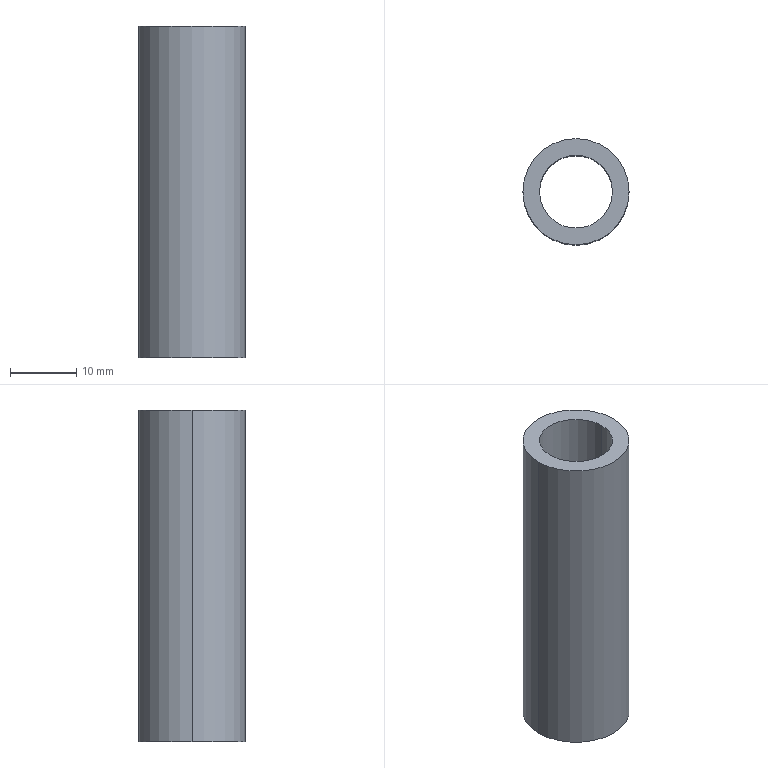Part | SolidWorks | features BaseBody 1 | 1 solid | 6 faces | box 16 x 16 x 50 mm | volume 5301 mm3 | cylinder 4 | plane 2 | commonest cylinder face diameters 11 x2 16 x2
STEP:
#1=CARTESIAN_POINT('',(-5.5,0.,-50.));
#2=VERTEX_POINT('',#1);
#3=CARTESIAN_POINT('',(-5.5,0.,0.));
#4=VERTEX_POINT('',#3);
#5=CARTESIAN_POINT('',(-5.5,0.,-50.));
#6=DIRECTION('',(0.,0.,1.));
#7=VECTOR('',#6,1000.);
#8=LINE('',#5,#7);
#9=EDGE_CURVE('',#2,#4,#8,.T.);
#10=ORIENTED_EDGE('',*,*,#9,.F.);
#11=CARTESIAN_POINT('',(5.5,0.,-50.));
#12=VERTEX_POINT('',#11);
#13=CARTESIAN_POINT('',(0.,0.,-50.));
#14=DIRECTION('',(0.,0.,1.));
#15=DIRECTION('',(1.,0.,0.));
#16=AXIS2_PLACEMENT_3D('',#13,#14,#15);
#17=CIRCLE('',#16,5.5);
#18=EDGE_CURVE('',#12,#2,#17,.T.);
#19=ORIENTED_EDGE('',*,*,#18,.F.);
#20=CARTESIAN_POINT('',(5.5,0.,0.));
#21=VERTEX_POINT('',#20);
#22=CARTESIAN_POINT('',(5.5,0.,-50.));
#23=DIRECTION('',(0.,0.,1.));
#24=VECTOR('',#23,1000.);
#25=LINE('',#22,#24);
#26=EDGE_CURVE('',#12,#21,#25,.T.);
#27=ORIENTED_EDGE('',*,*,#26,.T.);
#28=CARTESIAN_POINT('',(0.,0.,0.));
#29=DIRECTION('',(0.,0.,1.));
#30=DIRECTION('',(1.,0.,0.));
#31=AXIS2_PLACEMENT_3D('',#28,#29,#30);
#32=CIRCLE('',#31,5.5);
#33=EDGE_CURVE('',#21,#4,#32,.T.);
#34=ORIENTED_EDGE('',*,*,#33,.T.);
#35=EDGE_LOOP('',(#10,#19,#27,#34));
#36=FACE_OUTER_BOUND('',#35,.T.);
#37=CARTESIAN_POINT('',(0.,0.,-50.));
#38=DIRECTION('',(0.,0.,1.));
#39=DIRECTION('',(1.,0.,0.));
#40=AXIS2_PLACEMENT_3D('',#37,#38,#39);
#41=CYLINDRICAL_SURFACE('',#40,5.5);
#42=ADVANCED_FACE('',(#36),#41,.F.);
#43=ORIENTED_EDGE('',*,*,#33,.F.);
#44=CARTESIAN_POINT('',(0.,0.,0.));
#45=DIRECTION('',(0.,0.,1.));
#46=DIRECTION('',(1.,0.,0.));
#47=AXIS2_PLACEMENT_3D('',#44,#45,#46);
#48=CIRCLE('',#47,5.5);
#49=EDGE_CURVE('',#4,#21,#48,.T.);
#50=ORIENTED_EDGE('',*,*,#49,.F.);
#51=EDGE_LOOP('',(#43,#50));
#52=FACE_BOUND('',#51,.T.);
#53=CARTESIAN_POINT('',(8.,0.,0.));
#54=VERTEX_POINT('',#53);
#55=CARTESIAN_POINT('',(-8.,0.,0.));
#56=VERTEX_POINT('',#55);
#57=CARTESIAN_POINT('',(0.,0.,0.));
#58=DIRECTION('',(0.,0.,1.));
#59=DIRECTION('',(1.,0.,0.));
#60=AXIS2_PLACEMENT_3D('',#57,#58,#59);
#61=CIRCLE('',#60,8.);
#62=EDGE_CURVE('',#54,#56,#61,.T.);
#63=ORIENTED_EDGE('',*,*,#62,.T.);
#64=CARTESIAN_POINT('',(0.,0.,0.));
#65=DIRECTION('',(0.,0.,1.));
#66=DIRECTION('',(1.,0.,0.));
#67=AXIS2_PLACEMENT_3D('',#64,#65,#66);
#68=CIRCLE('',#67,8.);
#69=EDGE_CURVE('',#56,#54,#68,.T.);
#70=ORIENTED_EDGE('',*,*,#69,.T.);
#71=EDGE_LOOP('',(#63,#70));
#72=FACE_OUTER_BOUND('',#71,.T.);
#73=CARTESIAN_POINT('',(0.,0.,0.));
#74=DIRECTION('',(0.,0.,1.));
#75=DIRECTION('',(1.,0.,0.));
#76=AXIS2_PLACEMENT_3D('',#73,#74,#75);
#77=PLANE('',#76);
#78=ADVANCED_FACE('',(#52,#72),#77,.T.);
#79=ORIENTED_EDGE('',*,*,#18,.T.);
#80=CARTESIAN_POINT('',(0.,0.,-50.));
#81=DIRECTION('',(0.,0.,1.));
#82=DIRECTION('',(1.,0.,0.));
#83=AXIS2_PLACEMENT_3D('',#80,#81,#82);
#84=CIRCLE('',#83,5.5);
#85=EDGE_CURVE('',#2,#12,#84,.T.);
#86=ORIENTED_EDGE('',*,*,#85,.T.);
#87=EDGE_LOOP('',(#79,#86));
#88=FACE_BOUND('',#87,.T.);
#89=CARTESIAN_POINT('',(8.,0.,-50.));
#90=VERTEX_POINT('',#89);
#91=CARTESIAN_POINT('',(-8.,0.,-50.));
#92=VERTEX_POINT('',#91);
#93=CARTESIAN_POINT('',(0.,0.,-50.));
#94=DIRECTION('',(0.,0.,1.));
#95=DIRECTION('',(1.,0.,0.));
#96=AXIS2_PLACEMENT_3D('',#93,#94,#95);
#97=CIRCLE('',#96,8.);
#98=EDGE_CURVE('',#90,#92,#97,.T.);
#99=ORIENTED_EDGE('',*,*,#98,.F.);
#100=CARTESIAN_POINT('',(0.,0.,-50.));
#101=DIRECTION('',(0.,0.,1.));
#102=DIRECTION('',(1.,0.,0.));
#103=AXIS2_PLACEMENT_3D('',#100,#101,#102);
#104=CIRCLE('',#103,8.);
#105=EDGE_CURVE('',#92,#90,#104,.T.);
#106=ORIENTED_EDGE('',*,*,#105,.F.);
#107=EDGE_LOOP('',(#99,#106));
#108=FACE_OUTER_BOUND('',#107,.T.);
#109=CARTESIAN_POINT('',(0.,0.,-50.));
#110=DIRECTION('',(0.,0.,1.));
#111=DIRECTION('',(1.,0.,0.));
#112=AXIS2_PLACEMENT_3D('',#109,#110,#111);
#113=PLANE('',#112);
#114=ADVANCED_FACE('',(#88,#108),#113,.F.);
#115=CARTESIAN_POINT('',(-8.,0.,-50.));
#116=DIRECTION('',(0.,0.,1.));
#117=VECTOR('',#116,1000.);
#118=LINE('',#115,#117);
#119=EDGE_CURVE('',#92,#56,#118,.T.);
#120=ORIENTED_EDGE('',*,*,#119,.F.);
#121=ORIENTED_EDGE('',*,*,#105,.T.);
#122=CARTESIAN_POINT('',(8.,0.,-50.));
#123=DIRECTION('',(0.,0.,1.));
#124=VECTOR('',#123,1000.);
#125=LINE('',#122,#124);
#126=EDGE_CURVE('',#90,#54,#125,.T.);
#127=ORIENTED_EDGE('',*,*,#126,.T.);
#128=ORIENTED_EDGE('',*,*,#69,.F.);
#129=EDGE_LOOP('',(#120,#121,#127,#128));
#130=FACE_OUTER_BOUND('',#129,.T.);
#131=CARTESIAN_POINT('',(0.,0.,-50.));
#132=DIRECTION('',(0.,0.,1.));
#133=DIRECTION('',(1.,0.,0.));
#134=AXIS2_PLACEMENT_3D('',#131,#132,#133);
#135=CYLINDRICAL_SURFACE('',#134,8.);
#136=ADVANCED_FACE('',(#130),#135,.T.);
#137=ORIENTED_EDGE('',*,*,#98,.T.);
#138=ORIENTED_EDGE('',*,*,#119,.T.);
#139=ORIENTED_EDGE('',*,*,#62,.F.);
#140=ORIENTED_EDGE('',*,*,#126,.F.);
#141=EDGE_LOOP('',(#137,#138,#139,#140));
#142=FACE_OUTER_BOUND('',#141,.T.);
#143=CARTESIAN_POINT('',(0.,0.,-50.));
#144=DIRECTION('',(0.,0.,1.));
#145=DIRECTION('',(1.,0.,0.));
#146=AXIS2_PLACEMENT_3D('',#143,#144,#145);
#147=CYLINDRICAL_SURFACE('',#146,8.);
#148=ADVANCED_FACE('',(#142),#147,.T.);
#149=ORIENTED_EDGE('',*,*,#85,.F.);
#150=ORIENTED_EDGE('',*,*,#9,.T.);
#151=ORIENTED_EDGE('',*,*,#49,.T.);
#152=ORIENTED_EDGE('',*,*,#26,.F.);
#153=EDGE_LOOP('',(#149,#150,#151,#152));
#154=FACE_OUTER_BOUND('',#153,.T.);
#155=CARTESIAN_POINT('',(0.,0.,-50.));
#156=DIRECTION('',(0.,0.,1.));
#157=DIRECTION('',(1.,0.,0.));
#158=AXIS2_PLACEMENT_3D('',#155,#156,#157);
#159=CYLINDRICAL_SURFACE('',#158,5.5);
#160=ADVANCED_FACE('',(#154),#159,.F.);
#161=CLOSED_SHELL('',(#42,#78,#114,#136,#148,#160));
#162=MANIFOLD_SOLID_BREP('',#161);
#163=CARTESIAN_POINT('',(0.,0.,0.));
#164=DIRECTION('',(0.,0.,1.));
#165=DIRECTION('',(1.,0.,0.));
#166=AXIS2_PLACEMENT_3D('',#163,#164,#165);
#167=(LENGTH_UNIT()NAMED_UNIT(*)SI_UNIT(.MILLI.,.METRE.));
#168=UNCERTAINTY_MEASURE_WITH_UNIT(LENGTH_MEASURE(0.00001),#167,'','');
#169=(NAMED_UNIT(*)PLANE_ANGLE_UNIT()SI_UNIT($,.RADIAN.));
#170=(NAMED_UNIT(*)SI_UNIT($,.STERADIAN.)SOLID_ANGLE_UNIT());
#171=(GEOMETRIC_REPRESENTATION_CONTEXT(3)GLOBAL_UNCERTAINTY_ASSIGNED_CONTEXT((#168))GLOBAL_UNIT_ASSIGNED_CONTEXT((#167,#169,#170))REPRESENTATION_CONTEXT('',''));
#172=ADVANCED_BREP_SHAPE_REPRESENTATION('',(#162,#166),#171);